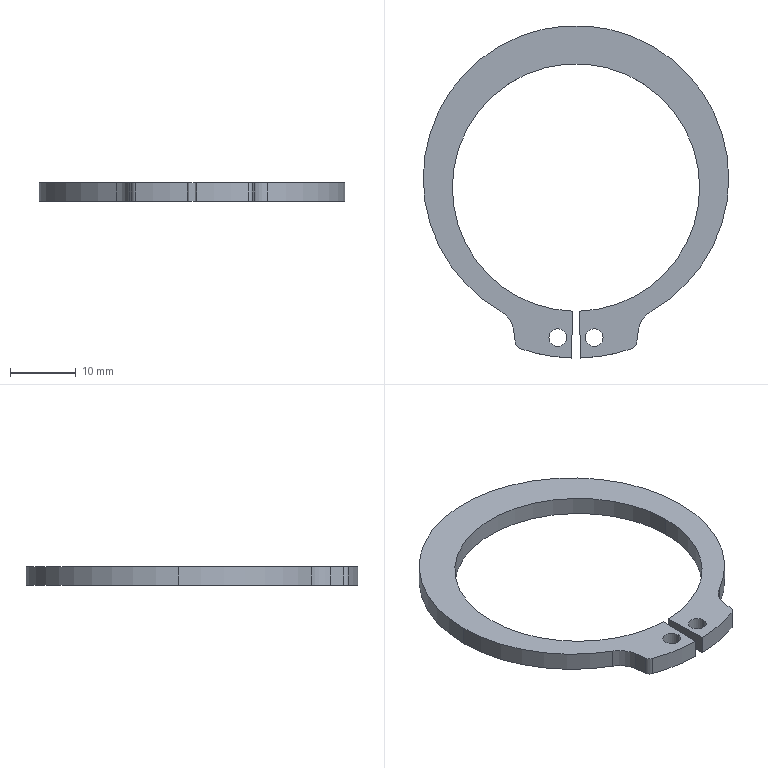Part | STEP file | heavy duty external retaining ring_am_B27.8M - 3DM1-40 | 1 solid | 22 faces | box 46.312 x 50.391 x 2.8 mm | volume 1790 mm3 | cylinder 16 | plane 6 | commonest cylinder face diameters 2.7 x4 37.5 x3 46.312 x3 2 x2 7.797 x2 51.7 x2